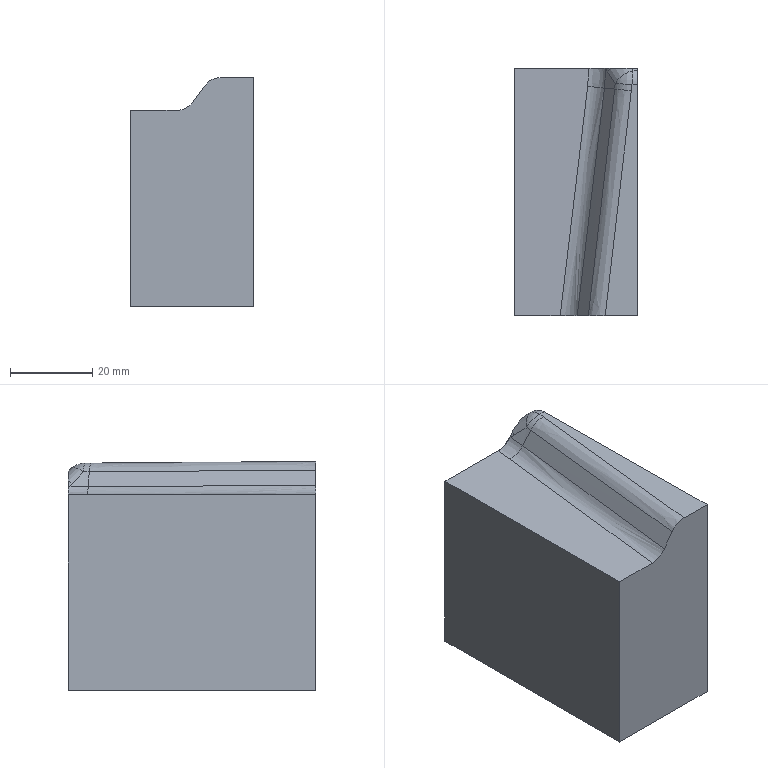Part | NX | features solid 2 | 1 solid | 19 faces | box 30 x 60 x 55.625 mm | volume 90245 mm3 | spline 14 | plane 5
STEP:
#1=CARTESIAN_POINT('',(-115.283,294.27,47.484));
#2=VERTEX_POINT('',#1);
#3=CARTESIAN_POINT('',(-133.378,294.27,47.551));
#4=VERTEX_POINT('',#3);
#5=CARTESIAN_POINT('',(-103.184,294.27,47.439));
#6=DIRECTION('',(-1.,0.,0.003698));
#7=VECTOR('',#6,1000.);
#8=LINE('',#5,#7);
#9=EDGE_CURVE('',#2,#4,#8,.T.);
#10=ORIENTED_EDGE('',*,*,#9,.F.);
#11=CARTESIAN_POINT('',(-111.203,294.27,49.568));
#12=VERTEX_POINT('',#11);
#13=CARTESIAN_POINT('',(-115.284,294.27,47.484));
#14=CARTESIAN_POINT('',(-113.684,294.27,47.478));
#15=CARTESIAN_POINT('',(-112.137,294.27,48.268));
#16=CARTESIAN_POINT('',(-111.203,294.27,49.568));
#17=B_SPLINE_CURVE_WITH_KNOTS('',3,(#13,#14,#15,#16),.UNSPECIFIED.,.F.,.F.,(4,4),(0.,0.004736),.UNSPECIFIED.);
#18=EDGE_CURVE('',#2,#12,#17,.T.);
#19=ORIENTED_EDGE('',*,*,#18,.T.);
#20=CARTESIAN_POINT('',(-110.093,294.27,50.867));
#21=VERTEX_POINT('',#20);
#22=CARTESIAN_POINT('',(-110.093,294.27,50.867));
#23=CARTESIAN_POINT('',(-110.496,294.27,50.461));
#24=CARTESIAN_POINT('',(-110.87,294.27,50.032));
#25=CARTESIAN_POINT('',(-111.203,294.27,49.568));
#26=B_SPLINE_CURVE_WITH_KNOTS('',3,(#22,#23,#24,#25),.UNSPECIFIED.,.F.,.F.,(4,4),(0.,0.001709),.UNSPECIFIED.);
#27=EDGE_CURVE('',#21,#12,#26,.T.);
#28=ORIENTED_EDGE('',*,*,#27,.F.);
#29=CARTESIAN_POINT('',(-104.912,294.27,53.297));
#30=VERTEX_POINT('',#29);
#31=CARTESIAN_POINT('',(-110.093,294.27,50.867));
#32=CARTESIAN_POINT('',(-109.399,294.27,51.567));
#33=CARTESIAN_POINT('',(-107.835,294.27,52.779));
#34=CARTESIAN_POINT('',(-105.906,294.27,53.356));
#35=CARTESIAN_POINT('',(-104.912,294.27,53.297));
#36=B_SPLINE_CURVE_WITH_KNOTS('',3,(#31,#32,#33,#34,#35),.UNSPECIFIED.,.F.,.F.,(4,1,4),(0.,0.00295,0.0059),.UNSPECIFIED.);
#37=EDGE_CURVE('',#21,#30,#36,.T.);
#38=ORIENTED_EDGE('',*,*,#37,.T.);
#39=CARTESIAN_POINT('',(-103.378,294.27,53.207));
#40=VERTEX_POINT('',#39);
#41=CARTESIAN_POINT('',(-99.969,294.27,53.007));
#42=DIRECTION('',(0.9983,0.,-0.05867));
#43=VECTOR('',#42,1000.);
#44=LINE('',#41,#43);
#45=EDGE_CURVE('',#30,#40,#44,.T.);
#46=ORIENTED_EDGE('',*,*,#45,.T.);
#47=CARTESIAN_POINT('',(-103.378,294.27,0.));
#48=VERTEX_POINT('',#47);
#49=CARTESIAN_POINT('',(-103.378,294.27,-5.));
#50=DIRECTION('',(0.,0.,-1.));
#51=VECTOR('',#50,1000.);
#52=LINE('',#49,#51);
#53=EDGE_CURVE('',#48,#40,#52,.F.);
#54=ORIENTED_EDGE('',*,*,#53,.F.);
#55=CARTESIAN_POINT('',(-133.378,294.27,0.));
#56=VERTEX_POINT('',#55);
#57=CARTESIAN_POINT('',(-103.378,294.27,0.));
#58=DIRECTION('',(1.,0.,0.));
#59=VECTOR('',#58,1000.);
#60=LINE('',#57,#59);
#61=EDGE_CURVE('',#48,#56,#60,.F.);
#62=ORIENTED_EDGE('',*,*,#61,.T.);
#63=CARTESIAN_POINT('',(-133.378,294.27,-5.));
#64=DIRECTION('',(0.,0.,-1.));
#65=VECTOR('',#64,1000.);
#66=LINE('',#63,#65);
#67=EDGE_CURVE('',#56,#4,#66,.F.);
#68=ORIENTED_EDGE('',*,*,#67,.T.);
#69=EDGE_LOOP('',(#10,#19,#28,#38,#46,#54,#62,#68));
#70=FACE_BOUND('',#69,.T.);
#71=CARTESIAN_POINT('',(-103.378,294.27,-5.));
#72=DIRECTION('',(0.,1.,0.));
#73=DIRECTION('',(-1.,0.,0.));
#74=AXIS2_PLACEMENT_3D('',#71,#72,#73);
#75=PLANE('',#74);
#76=ADVANCED_FACE('',(#70),#75,.T.);
#77=CARTESIAN_POINT('',(-133.378,234.27,47.656));
#78=VERTEX_POINT('',#77);
#79=CARTESIAN_POINT('',(-122.215,234.27,47.614));
#80=VERTEX_POINT('',#79);
#81=CARTESIAN_POINT('',(-103.184,234.27,47.544));
#82=DIRECTION('',(-1.,0.,0.003698));
#83=VECTOR('',#82,1000.);
#84=LINE('',#81,#83);
#85=EDGE_CURVE('',#78,#80,#84,.F.);
#86=ORIENTED_EDGE('',*,*,#85,.F.);
#87=CARTESIAN_POINT('',(-133.378,234.27,0.));
#88=VERTEX_POINT('',#87);
#89=CARTESIAN_POINT('',(-133.378,234.27,-5.));
#90=DIRECTION('',(0.,0.,-1.));
#91=VECTOR('',#90,1000.);
#92=LINE('',#89,#91);
#93=EDGE_CURVE('',#88,#78,#92,.F.);
#94=ORIENTED_EDGE('',*,*,#93,.F.);
#95=CARTESIAN_POINT('',(-103.378,234.27,0.));
#96=VERTEX_POINT('',#95);
#97=CARTESIAN_POINT('',(-103.378,234.27,0.));
#98=DIRECTION('',(-1.,0.,0.));
#99=VECTOR('',#98,1000.);
#100=LINE('',#97,#99);
#101=EDGE_CURVE('',#96,#88,#100,.T.);
#102=ORIENTED_EDGE('',*,*,#101,.F.);
#103=CARTESIAN_POINT('',(-103.378,234.27,55.625));
#104=VERTEX_POINT('',#103);
#105=CARTESIAN_POINT('',(-103.378,234.27,-5.));
#106=DIRECTION('',(0.,0.,-1.));
#107=VECTOR('',#106,1000.);
#108=LINE('',#105,#107);
#109=EDGE_CURVE('',#96,#104,#108,.F.);
#110=ORIENTED_EDGE('',*,*,#109,.T.);
#111=CARTESIAN_POINT('',(-111.283,234.27,55.625));
#112=VERTEX_POINT('',#111);
#113=CARTESIAN_POINT('',(-103.378,234.27,55.625));
#114=DIRECTION('',(1.,0.,0.));
#115=VECTOR('',#114,1000.);
#116=LINE('',#113,#115);
#117=EDGE_CURVE('',#104,#112,#116,.F.);
#118=ORIENTED_EDGE('',*,*,#117,.T.);
#119=CARTESIAN_POINT('',(-115.39,234.27,53.514));
#120=VERTEX_POINT('',#119);
#121=CARTESIAN_POINT('',(-111.283,234.27,55.625));
#122=CARTESIAN_POINT('',(-112.896,234.27,55.625));
#123=CARTESIAN_POINT('',(-114.454,234.27,54.829));
#124=CARTESIAN_POINT('',(-115.39,234.27,53.514));
#125=B_SPLINE_CURVE_WITH_KNOTS('',3,(#121,#122,#123,#124),.UNSPECIFIED.,.F.,.F.,(4,4),(0.,0.004803),.UNSPECIFIED.);
#126=EDGE_CURVE('',#112,#120,#125,.T.);
#127=ORIENTED_EDGE('',*,*,#126,.T.);
#128=CARTESIAN_POINT('',(-118.085,234.27,49.728));
#129=VERTEX_POINT('',#128);
#130=CARTESIAN_POINT('',(-138.995,234.27,20.355));
#131=DIRECTION('',(-0.5799,0.,-0.8147));
#132=VECTOR('',#131,1000.);
#133=LINE('',#130,#132);
#134=EDGE_CURVE('',#129,#120,#133,.F.);
#135=ORIENTED_EDGE('',*,*,#134,.F.);
#136=CARTESIAN_POINT('',(-122.215,234.27,47.614));
#137=CARTESIAN_POINT('',(-120.594,234.27,47.608));
#138=CARTESIAN_POINT('',(-119.026,234.27,48.407));
#139=CARTESIAN_POINT('',(-118.085,234.27,49.728));
#140=B_SPLINE_CURVE_WITH_KNOTS('',3,(#136,#137,#138,#139),.UNSPECIFIED.,.F.,.F.,(4,4),(0.,0.004827),.UNSPECIFIED.);
#141=EDGE_CURVE('',#80,#129,#140,.T.);
#142=ORIENTED_EDGE('',*,*,#141,.F.);
#143=EDGE_LOOP('',(#86,#94,#102,#110,#118,#127,#135,#142));
#144=FACE_BOUND('',#143,.T.);
#145=CARTESIAN_POINT('',(-103.378,234.27,-5.));
#146=DIRECTION('',(0.,1.,0.));
#147=DIRECTION('',(-1.,0.,0.));
#148=AXIS2_PLACEMENT_3D('',#145,#146,#147);
#149=PLANE('',#148);
#150=ADVANCED_FACE('',(#144),#149,.F.);
#151=CARTESIAN_POINT('',(-133.378,294.362,47.551));
#152=DIRECTION('',(0.,-1.,0.00175));
#153=VECTOR('',#152,1000.);
#154=LINE('',#151,#153);
#155=EDGE_CURVE('',#4,#78,#154,.T.);
#156=ORIENTED_EDGE('',*,*,#155,.F.);
#157=ORIENTED_EDGE('',*,*,#67,.F.);
#158=CARTESIAN_POINT('',(-133.378,294.27,0.));
#159=DIRECTION('',(0.,1.,0.));
#160=VECTOR('',#159,1000.);
#161=LINE('',#158,#160);
#162=EDGE_CURVE('',#56,#88,#161,.F.);
#163=ORIENTED_EDGE('',*,*,#162,.T.);
#164=ORIENTED_EDGE('',*,*,#93,.T.);
#165=EDGE_LOOP('',(#156,#157,#163,#164));
#166=FACE_BOUND('',#165,.T.);
#167=CARTESIAN_POINT('',(-133.378,294.27,-5.));
#168=DIRECTION('',(-1.,0.,0.));
#169=DIRECTION('',(0.,-1.,0.));
#170=AXIS2_PLACEMENT_3D('',#167,#168,#169);
#171=PLANE('',#170);
#172=ADVANCED_FACE('',(#166),#171,.T.);
#173=CARTESIAN_POINT('',(-103.378,293.627,53.826));
#174=VERTEX_POINT('',#173);
#175=CARTESIAN_POINT('',(-103.378,290.188,55.224));
#176=VERTEX_POINT('',#175);
#177=CARTESIAN_POINT('',(-103.378,293.627,53.826));
#178=CARTESIAN_POINT('',(-103.378,292.707,54.71));
#179=CARTESIAN_POINT('',(-103.378,291.464,55.215));
#180=CARTESIAN_POINT('',(-103.378,290.188,55.224));
#181=B_SPLINE_CURVE_WITH_KNOTS('',3,(#177,#178,#179,#180),.UNSPECIFIED.,.F.,.F.,(4,4),(0.,0.003809),.UNSPECIFIED.);
#182=EDGE_CURVE('',#174,#176,#181,.T.);
#183=ORIENTED_EDGE('',*,*,#182,.T.);
#184=CARTESIAN_POINT('',(-103.378,294.703,55.192));
#185=DIRECTION('',(0.,1.,-0.007178));
#186=VECTOR('',#185,1000.);
#187=LINE('',#184,#186);
#188=EDGE_CURVE('',#176,#104,#187,.F.);
#189=ORIENTED_EDGE('',*,*,#188,.T.);
#190=ORIENTED_EDGE('',*,*,#109,.F.);
#191=CARTESIAN_POINT('',(-103.378,294.27,0.));
#192=DIRECTION('',(0.,-1.,0.));
#193=VECTOR('',#192,1000.);
#194=LINE('',#191,#193);
#195=EDGE_CURVE('',#48,#96,#194,.T.);
#196=ORIENTED_EDGE('',*,*,#195,.F.);
#197=ORIENTED_EDGE('',*,*,#53,.T.);
#198=CARTESIAN_POINT('',(-103.378,323.351,25.253));
#199=DIRECTION('',(0.,0.7209,-0.693));
#200=VECTOR('',#199,1000.);
#201=LINE('',#198,#200);
#202=EDGE_CURVE('',#40,#174,#201,.F.);
#203=ORIENTED_EDGE('',*,*,#202,.T.);
#204=EDGE_LOOP('',(#183,#189,#190,#196,#197,#203));
#205=FACE_BOUND('',#204,.T.);
#206=CARTESIAN_POINT('',(-103.378,294.27,-5.));
#207=DIRECTION('',(-1.,0.,0.));
#208=DIRECTION('',(0.,-1.,0.));
#209=AXIS2_PLACEMENT_3D('',#206,#207,#208);
#210=PLANE('',#209);
#211=ADVANCED_FACE('',(#205),#210,.F.);
#212=ORIENTED_EDGE('',*,*,#101,.T.);
#213=ORIENTED_EDGE('',*,*,#162,.F.);
#214=ORIENTED_EDGE('',*,*,#61,.F.);
#215=ORIENTED_EDGE('',*,*,#195,.T.);
#216=EDGE_LOOP('',(#212,#213,#214,#215));
#217=FACE_BOUND('',#216,.T.);
#218=CARTESIAN_POINT('',(-103.378,294.27,0.));
#219=DIRECTION('',(0.,0.,1.));
#220=DIRECTION('',(1.,0.,0.));
#221=AXIS2_PLACEMENT_3D('',#218,#219,#220);
#222=PLANE('',#221);
#223=ADVANCED_FACE('',(#217),#222,.F.);
#224=CARTESIAN_POINT('',(-115.285,294.158,47.484));
#225=VERTEX_POINT('',#224);
#226=CARTESIAN_POINT('',(-115.284,294.27,47.484));
#227=CARTESIAN_POINT('',(-115.284,294.233,47.484));
#228=CARTESIAN_POINT('',(-115.285,294.195,47.484));
#229=CARTESIAN_POINT('',(-115.285,294.158,47.484));
#230=B_SPLINE_CURVE_WITH_KNOTS('',3,(#226,#227,#228,#229),.UNSPECIFIED.,.F.,.F.,(4,4),(0.965,1.),.UNSPECIFIED.);
#231=EDGE_CURVE('',#2,#225,#230,.T.);
#232=ORIENTED_EDGE('',*,*,#231,.T.);
#233=CARTESIAN_POINT('',(-111.18,294.144,49.603));
#234=VERTEX_POINT('',#233);
#235=CARTESIAN_POINT('',(-115.285,294.158,47.484));
#236=CARTESIAN_POINT('',(-113.684,294.151,47.478));
#237=CARTESIAN_POINT('',(-112.102,294.146,48.295));
#238=CARTESIAN_POINT('',(-111.18,294.144,49.603));
#239=B_SPLINE_CURVE_WITH_KNOTS('',3,(#235,#236,#237,#238),.UNSPECIFIED.,.F.,.F.,(4,4),(0.,1.),.UNSPECIFIED.);
#240=EDGE_CURVE('',#234,#225,#239,.F.);
#241=ORIENTED_EDGE('',*,*,#240,.F.);
#242=CARTESIAN_POINT('',(-111.18,294.144,49.603));
#243=CARTESIAN_POINT('',(-111.188,294.186,49.591));
#244=CARTESIAN_POINT('',(-111.196,294.228,49.58));
#245=CARTESIAN_POINT('',(-111.203,294.27,49.568));
#246=B_SPLINE_CURVE_WITH_KNOTS('',3,(#242,#243,#244,#245),.UNSPECIFIED.,.F.,.F.,(4,4),(0.,0.04789),.UNSPECIFIED.);
#247=EDGE_CURVE('',#234,#12,#246,.T.);
#248=ORIENTED_EDGE('',*,*,#247,.T.);
#249=ORIENTED_EDGE('',*,*,#18,.F.);
#250=EDGE_LOOP('',(#232,#241,#248,#249));
#251=FACE_BOUND('',#250,.T.);
#252=CARTESIAN_POINT('',(-115.283,294.313,47.484));
#253=CARTESIAN_POINT('',(-114.332,294.302,47.48));
#254=CARTESIAN_POINT('',(-113.379,294.292,47.703));
#255=CARTESIAN_POINT('',(-112.498,294.283,48.154));
#256=CARTESIAN_POINT('',(-111.759,294.276,48.795));
#257=CARTESIAN_POINT('',(-111.204,294.271,49.568));
#258=CARTESIAN_POINT('',(-115.284,294.282,47.484));
#259=CARTESIAN_POINT('',(-114.33,294.273,47.48));
#260=CARTESIAN_POINT('',(-113.376,294.264,47.704));
#261=CARTESIAN_POINT('',(-112.493,294.256,48.156));
#262=CARTESIAN_POINT('',(-111.754,294.25,48.799));
#263=CARTESIAN_POINT('',(-111.199,294.246,49.575));
#264=CARTESIAN_POINT('',(-115.284,294.251,47.484));
#265=CARTESIAN_POINT('',(-114.329,294.243,47.48));
#266=CARTESIAN_POINT('',(-113.373,294.235,47.705));
#267=CARTESIAN_POINT('',(-112.489,294.229,48.158));
#268=CARTESIAN_POINT('',(-111.749,294.224,48.804));
#269=CARTESIAN_POINT('',(-111.194,294.22,49.582));
#270=CARTESIAN_POINT('',(-115.284,294.22,47.484));
#271=CARTESIAN_POINT('',(-114.327,294.213,47.48));
#272=CARTESIAN_POINT('',(-113.37,294.207,47.706));
#273=CARTESIAN_POINT('',(-112.484,294.202,48.161));
#274=CARTESIAN_POINT('',(-111.743,294.198,48.809));
#275=CARTESIAN_POINT('',(-111.189,294.195,49.589));
#276=CARTESIAN_POINT('',(-115.285,294.189,47.484));
#277=CARTESIAN_POINT('',(-114.326,294.183,47.48));
#278=CARTESIAN_POINT('',(-113.366,294.179,47.707));
#279=CARTESIAN_POINT('',(-112.48,294.174,48.163));
#280=CARTESIAN_POINT('',(-111.738,294.171,48.813));
#281=CARTESIAN_POINT('',(-111.185,294.17,49.596));
#282=CARTESIAN_POINT('',(-115.285,294.158,47.484));
#283=CARTESIAN_POINT('',(-114.324,294.154,47.481));
#284=CARTESIAN_POINT('',(-113.363,294.15,47.708));
#285=CARTESIAN_POINT('',(-112.475,294.147,48.166));
#286=CARTESIAN_POINT('',(-111.733,294.145,48.818));
#287=CARTESIAN_POINT('',(-111.18,294.144,49.603));
#288=B_SPLINE_SURFACE_WITH_KNOTS('',5,5,((#252,#253,#254,#255,#256,#257),(#258,#259,#260,#261,#262,#263),(#264,#265,#266,#267,#268,#269),(#270,#271,#272,#273,#274,#275),(#276,#277,#278,#279,#280,#281),(#282,#283,#284,#285,#286,#287)),.UNSPECIFIED.,.F.,.F.,.F.,(6,6),(6,6),(0.9518,1.),(0.,1.),.PIECEWISE_BEZIER_KNOTS.);
#289=ADVANCED_FACE('',(#251),#288,.T.);
#290=ORIENTED_EDGE('',*,*,#27,.T.);
#291=ORIENTED_EDGE('',*,*,#247,.F.);
#292=CARTESIAN_POINT('',(-110.699,293.366,50.301));
#293=VERTEX_POINT('',#292);
#294=CARTESIAN_POINT('',(-110.699,293.366,50.301));
#295=CARTESIAN_POINT('',(-110.866,293.608,50.056));
#296=CARTESIAN_POINT('',(-111.027,293.867,49.822));
#297=CARTESIAN_POINT('',(-111.18,294.144,49.603));
#298=B_SPLINE_CURVE_WITH_KNOTS('',3,(#294,#295,#296,#297),.UNSPECIFIED.,.F.,.F.,(4,4),(0.,1.),.UNSPECIFIED.);
#299=EDGE_CURVE('',#293,#234,#298,.T.);
#300=ORIENTED_EDGE('',*,*,#299,.F.);
#301=CARTESIAN_POINT('',(-110.093,294.27,50.867));
#302=CARTESIAN_POINT('',(-110.332,293.976,50.711));
#303=CARTESIAN_POINT('',(-110.536,293.671,50.52));
#304=CARTESIAN_POINT('',(-110.699,293.366,50.301));
#305=B_SPLINE_CURVE_WITH_KNOTS('',3,(#301,#302,#303,#304),.UNSPECIFIED.,.F.,.F.,(4,4),(0.7889,1.),.UNSPECIFIED.);
#306=EDGE_CURVE('',#21,#293,#305,.T.);
#307=ORIENTED_EDGE('',*,*,#306,.F.);
#308=EDGE_LOOP('',(#290,#291,#300,#307));
#309=FACE_BOUND('',#308,.T.);
#310=CARTESIAN_POINT('',(-110.593,295.007,50.184));
#311=CARTESIAN_POINT('',(-110.742,294.857,50.072));
#312=CARTESIAN_POINT('',(-110.881,294.704,49.95));
#313=CARTESIAN_POINT('',(-111.009,294.55,49.818));
#314=CARTESIAN_POINT('',(-111.126,294.395,49.678));
#315=CARTESIAN_POINT('',(-111.232,294.239,49.529));
#316=CARTESIAN_POINT('',(-110.498,294.849,50.312));
#317=CARTESIAN_POINT('',(-110.646,294.693,50.203));
#318=CARTESIAN_POINT('',(-110.783,294.534,50.085));
#319=CARTESIAN_POINT('',(-110.911,294.374,49.956));
#320=CARTESIAN_POINT('',(-111.027,294.213,49.819));
#321=CARTESIAN_POINT('',(-111.131,294.052,49.673));
#322=CARTESIAN_POINT('',(-110.399,294.697,50.445));
#323=CARTESIAN_POINT('',(-110.546,294.535,50.34));
#324=CARTESIAN_POINT('',(-110.683,294.371,50.225));
#325=CARTESIAN_POINT('',(-110.809,294.204,50.1));
#326=CARTESIAN_POINT('',(-110.924,294.037,49.965));
#327=CARTESIAN_POINT('',(-111.027,293.87,49.823));
#328=CARTESIAN_POINT('',(-110.298,294.55,50.583));
#329=CARTESIAN_POINT('',(-110.444,294.383,50.481));
#330=CARTESIAN_POINT('',(-110.58,294.213,50.37));
#331=CARTESIAN_POINT('',(-110.705,294.041,50.248));
#332=CARTESIAN_POINT('',(-110.819,293.869,50.117));
#333=CARTESIAN_POINT('',(-110.92,293.695,49.977));
#334=CARTESIAN_POINT('',(-110.195,294.41,50.724));
#335=CARTESIAN_POINT('',(-110.34,294.237,50.627));
#336=CARTESIAN_POINT('',(-110.475,294.062,50.519));
#337=CARTESIAN_POINT('',(-110.599,293.885,50.401));
#338=CARTESIAN_POINT('',(-110.711,293.706,50.273));
#339=CARTESIAN_POINT('',(-110.811,293.527,50.137));
#340=CARTESIAN_POINT('',(-110.089,294.276,50.87));
#341=CARTESIAN_POINT('',(-110.234,294.098,50.776));
#342=CARTESIAN_POINT('',(-110.368,293.917,50.672));
#343=CARTESIAN_POINT('',(-110.49,293.734,50.557));
#344=CARTESIAN_POINT('',(-110.601,293.55,50.433));
#345=CARTESIAN_POINT('',(-110.699,293.366,50.301));
#346=B_SPLINE_SURFACE_WITH_KNOTS('',5,5,((#310,#311,#312,#313,#314,#315),(#316,#317,#318,#319,#320,#321),(#322,#323,#324,#325,#326,#327),(#328,#329,#330,#331,#332,#333),(#334,#335,#336,#337,#338,#339),(#340,#341,#342,#343,#344,#345)),.UNSPECIFIED.,.F.,.F.,.F.,(6,6),(6,6),(0.6827,1.),(0.7877,1.),.PIECEWISE_BEZIER_KNOTS.);
#347=ADVANCED_FACE('',(#309),#346,.F.);
#348=ORIENTED_EDGE('',*,*,#306,.T.);
#349=CARTESIAN_POINT('',(-108.861,290.595,53.109));
#350=VERTEX_POINT('',#349);
#351=CARTESIAN_POINT('',(-110.699,293.366,50.301));
#352=CARTESIAN_POINT('',(-110.064,292.449,51.23));
#353=CARTESIAN_POINT('',(-109.452,291.526,52.166));
#354=CARTESIAN_POINT('',(-108.863,290.595,53.111));
#355=B_SPLINE_CURVE_WITH_KNOTS('',3,(#351,#352,#353,#354),.UNSPECIFIED.,.F.,.F.,(4,4),(0.,1.),.UNSPECIFIED.);
#356=EDGE_CURVE('',#350,#293,#355,.F.);
#357=ORIENTED_EDGE('',*,*,#356,.F.);
#358=CARTESIAN_POINT('',(-104.584,293.701,53.825));
#359=VERTEX_POINT('',#358);
#360=CARTESIAN_POINT('',(-108.863,290.595,53.111));
#361=CARTESIAN_POINT('',(-108.047,291.971,54.091));
#362=CARTESIAN_POINT('',(-106.313,293.229,54.38));
#363=CARTESIAN_POINT('',(-104.584,293.701,53.825));
#364=B_SPLINE_CURVE_WITH_KNOTS('',3,(#360,#361,#362,#363),.UNSPECIFIED.,.F.,.F.,(4,4),(0.,1.),.UNSPECIFIED.);
#365=EDGE_CURVE('',#350,#359,#364,.T.);
#366=ORIENTED_EDGE('',*,*,#365,.T.);
#367=CARTESIAN_POINT('',(-104.584,293.701,53.825));
#368=CARTESIAN_POINT('',(-104.693,293.891,53.649));
#369=CARTESIAN_POINT('',(-104.802,294.081,53.473));
#370=CARTESIAN_POINT('',(-104.912,294.27,53.297));
#371=B_SPLINE_CURVE_WITH_KNOTS('',3,(#367,#368,#369,#370),.UNSPECIFIED.,.F.,.F.,(4,4),(0.,0.1866),.UNSPECIFIED.);
#372=EDGE_CURVE('',#30,#359,#371,.F.);
#373=ORIENTED_EDGE('',*,*,#372,.F.);
#374=ORIENTED_EDGE('',*,*,#37,.F.);
#375=EDGE_LOOP('',(#348,#357,#366,#373,#374));
#376=FACE_BOUND('',#375,.T.);
#377=CARTESIAN_POINT('',(-104.584,293.701,53.825));
#378=CARTESIAN_POINT('',(-105.621,293.418,54.158));
#379=CARTESIAN_POINT('',(-106.672,292.916,54.263));
#380=CARTESIAN_POINT('',(-107.626,292.223,54.104));
#381=CARTESIAN_POINT('',(-108.373,291.421,53.699));
#382=CARTESIAN_POINT('',(-108.863,290.595,53.111));
#383=CARTESIAN_POINT('',(-104.933,294.312,53.258));
#384=CARTESIAN_POINT('',(-105.974,294.021,53.599));
#385=CARTESIAN_POINT('',(-107.029,293.508,53.709));
#386=CARTESIAN_POINT('',(-107.986,292.803,53.549));
#387=CARTESIAN_POINT('',(-108.732,291.988,53.139));
#388=CARTESIAN_POINT('',(-109.216,291.154,52.544));
#389=CARTESIAN_POINT('',(-105.29,294.921,52.695));
#390=CARTESIAN_POINT('',(-106.335,294.622,53.043));
#391=CARTESIAN_POINT('',(-107.394,294.098,53.157));
#392=CARTESIAN_POINT('',(-108.353,293.38,52.997));
#393=CARTESIAN_POINT('',(-109.097,292.553,52.582));
#394=CARTESIAN_POINT('',(-109.576,291.71,51.98));
#395=CARTESIAN_POINT('',(-105.654,295.527,52.133));
#396=CARTESIAN_POINT('',(-106.703,295.22,52.489));
#397=CARTESIAN_POINT('',(-107.766,294.685,52.608));
#398=CARTESIAN_POINT('',(-108.727,293.954,52.447));
#399=CARTESIAN_POINT('',(-109.47,293.116,52.028));
#400=CARTESIAN_POINT('',(-109.944,292.264,51.418));
#401=CARTESIAN_POINT('',(-106.025,296.131,51.574));
#402=CARTESIAN_POINT('',(-107.078,295.817,51.938));
#403=CARTESIAN_POINT('',(-108.146,295.27,52.061));
#404=CARTESIAN_POINT('',(-109.109,294.527,51.9));
#405=CARTESIAN_POINT('',(-109.85,293.676,51.476));
#406=CARTESIAN_POINT('',(-110.318,292.816,50.858));
#407=CARTESIAN_POINT('',(-106.404,296.732,51.018));
#408=CARTESIAN_POINT('',(-107.461,296.41,51.39));
#409=CARTESIAN_POINT('',(-108.532,295.853,51.517));
#410=CARTESIAN_POINT('',(-109.498,295.097,51.355));
#411=CARTESIAN_POINT('',(-110.237,294.235,50.926));
#412=CARTESIAN_POINT('',(-110.699,293.366,50.301));
#413=B_SPLINE_SURFACE_WITH_KNOTS('',5,5,((#377,#378,#379,#380,#381,#382),(#383,#384,#385,#386,#387,#388),(#389,#390,#391,#392,#393,#394),(#395,#396,#397,#398,#399,#400),(#401,#402,#403,#404,#405,#406),(#407,#408,#409,#410,#411,#412)),.UNSPECIFIED.,.F.,.F.,.F.,(6,6),(6,6),(0.,1.),(0.,1.),.PIECEWISE_BEZIER_KNOTS.);
#414=ADVANCED_FACE('',(#376),#413,.T.);
#415=ORIENTED_EDGE('',*,*,#372,.T.);
#416=CARTESIAN_POINT('',(-104.584,293.701,53.825));
#417=CARTESIAN_POINT('',(-104.182,293.677,53.825));
#418=CARTESIAN_POINT('',(-103.78,293.652,53.825));
#419=CARTESIAN_POINT('',(-103.378,293.627,53.826));
#420=B_SPLINE_CURVE_WITH_KNOTS('',3,(#416,#417,#418,#419),.UNSPECIFIED.,.F.,.F.,(4,4),(0.,0.02048),.UNSPECIFIED.);
#421=EDGE_CURVE('',#359,#174,#420,.T.);
#422=ORIENTED_EDGE('',*,*,#421,.T.);
#423=ORIENTED_EDGE('',*,*,#202,.F.);
#424=ORIENTED_EDGE('',*,*,#45,.F.);
#425=EDGE_LOOP('',(#415,#422,#423,#424));
#426=FACE_BOUND('',#425,.T.);
#427=CARTESIAN_POINT('',(-104.922,294.32,53.251));
#428=CARTESIAN_POINT('',(-103.378,294.274,53.203));
#429=CARTESIAN_POINT('',(-104.922,293.669,53.876));
#430=CARTESIAN_POINT('',(-103.378,293.623,53.829));
#431=B_SPLINE_SURFACE_WITH_KNOTS('',1,1,((#427,#428),(#429,#430)),.PLANE_SURF.,.F.,.F.,.F.,(2,2),(2,2),(0.551,0.6661),(0.03004,0.05514),.PIECEWISE_BEZIER_KNOTS.);
#432=ADVANCED_FACE('',(#426),#431,.T.);
#433=ORIENTED_EDGE('',*,*,#421,.F.);
#434=CARTESIAN_POINT('',(-104.796,290.275,55.222));
#435=VERTEX_POINT('',#434);
#436=CARTESIAN_POINT('',(-104.796,290.275,55.223));
#437=CARTESIAN_POINT('',(-104.72,291.509,55.215));
#438=CARTESIAN_POINT('',(-104.639,292.813,54.682));
#439=CARTESIAN_POINT('',(-104.584,293.701,53.825));
#440=B_SPLINE_CURVE_WITH_KNOTS('',3,(#436,#437,#438,#439),.UNSPECIFIED.,.F.,.F.,(4,4),(0.,1.),.UNSPECIFIED.);
#441=EDGE_CURVE('',#435,#359,#440,.T.);
#442=ORIENTED_EDGE('',*,*,#441,.F.);
#443=CARTESIAN_POINT('',(-103.378,290.188,55.224));
#444=CARTESIAN_POINT('',(-103.851,290.217,55.224));
#445=CARTESIAN_POINT('',(-104.323,290.246,55.224));
#446=CARTESIAN_POINT('',(-104.796,290.275,55.223));
#447=B_SPLINE_CURVE_WITH_KNOTS('',3,(#443,#444,#445,#446),.UNSPECIFIED.,.F.,.F.,(4,4),(0.7806,1.),.UNSPECIFIED.);
#448=EDGE_CURVE('',#176,#435,#447,.T.);
#449=ORIENTED_EDGE('',*,*,#448,.F.);
#450=ORIENTED_EDGE('',*,*,#182,.F.);
#451=EDGE_LOOP('',(#433,#442,#449,#450));
#452=FACE_BOUND('',#451,.T.);
#453=CARTESIAN_POINT('',(-104.796,290.275,55.223));
#454=CARTESIAN_POINT('',(-103.37,290.188,55.224));
#455=CARTESIAN_POINT('',(-104.716,291.57,55.214));
#456=CARTESIAN_POINT('',(-103.29,291.482,55.215));
#457=CARTESIAN_POINT('',(-104.642,292.769,54.725));
#458=CARTESIAN_POINT('',(-103.216,292.681,54.725));
#459=CARTESIAN_POINT('',(-104.584,293.701,53.825));
#460=CARTESIAN_POINT('',(-103.158,293.614,53.826));
#461=(BOUNDED_SURFACE()B_SPLINE_SURFACE(3,1,((#453,#454),(#455,#456),(#457,#458),(#459,#460)),.CYLINDRICAL_SURF.,.F.,.F.,.F.)B_SPLINE_SURFACE_WITH_KNOTS((4,4),(2,2),(0.,1.),(0.,0.02422),.PIECEWISE_BEZIER_KNOTS.)GEOMETRIC_REPRESENTATION_ITEM()RATIONAL_B_SPLINE_SURFACE(((1.,1.),(0.9525,0.9525),(0.9525,0.9525),(1.,1.)))REPRESENTATION_ITEM('')SURFACE());
#462=ADVANCED_FACE('',(#452),#461,.F.);
#463=ORIENTED_EDGE('',*,*,#141,.T.);
#464=CARTESIAN_POINT('',(-111.474,289.44,49.607));
#465=VERTEX_POINT('',#464);
#466=CARTESIAN_POINT('',(-118.085,234.27,49.728));
#467=CARTESIAN_POINT('',(-115.882,252.66,49.687));
#468=CARTESIAN_POINT('',(-113.678,271.05,49.647));
#469=CARTESIAN_POINT('',(-111.474,289.44,49.607));
#470=B_SPLINE_CURVE_WITH_KNOTS('',3,(#466,#467,#468,#469),.UNSPECIFIED.,.F.,.F.,(4,4),(0.4119,1.),.UNSPECIFIED.);
#471=EDGE_CURVE('',#465,#129,#470,.F.);
#472=ORIENTED_EDGE('',*,*,#471,.F.);
#473=CARTESIAN_POINT('',(-115.546,289.923,47.492));
#474=VERTEX_POINT('',#473);
#475=CARTESIAN_POINT('',(-111.474,289.44,49.607));
#476=CARTESIAN_POINT('',(-111.915,289.491,48.979));
#477=CARTESIAN_POINT('',(-113.159,289.638,47.862));
#478=CARTESIAN_POINT('',(-114.783,289.832,47.49));
#479=CARTESIAN_POINT('',(-115.546,289.923,47.492));
#480=B_SPLINE_CURVE_WITH_KNOTS('',3,(#475,#476,#477,#478,#479),.UNSPECIFIED.,.F.,.F.,(4,1,4),(0.,0.5,1.),.UNSPECIFIED.);
#481=EDGE_CURVE('',#474,#465,#480,.F.);
#482=ORIENTED_EDGE('',*,*,#481,.F.);
#483=CARTESIAN_POINT('',(-115.546,289.923,47.492));
#484=CARTESIAN_POINT('',(-117.769,271.372,47.533));
#485=CARTESIAN_POINT('',(-119.992,252.821,47.574));
#486=CARTESIAN_POINT('',(-122.215,234.27,47.614));
#487=B_SPLINE_CURVE_WITH_KNOTS('',3,(#483,#484,#485,#486),.UNSPECIFIED.,.F.,.F.,(4,4),(0.,0.5932),.UNSPECIFIED.);
#488=EDGE_CURVE('',#474,#80,#487,.T.);
#489=ORIENTED_EDGE('',*,*,#488,.T.);
#490=EDGE_LOOP('',(#463,#472,#482,#489));
#491=FACE_BOUND('',#490,.T.);
#492=CARTESIAN_POINT('',(-118.183,233.453,49.73));
#493=CARTESIAN_POINT('',(-111.474,289.44,49.607));
#494=CARTESIAN_POINT('',(-119.137,233.564,48.372));
#495=CARTESIAN_POINT('',(-112.427,289.551,48.249));
#496=CARTESIAN_POINT('',(-120.604,233.739,47.609));
#497=CARTESIAN_POINT('',(-113.895,289.725,47.487));
#498=CARTESIAN_POINT('',(-122.255,233.937,47.615));
#499=CARTESIAN_POINT('',(-115.546,289.923,47.492));
#500=(BOUNDED_SURFACE()B_SPLINE_SURFACE(3,1,((#492,#493),(#494,#495),(#496,#497),(#498,#499)),.CYLINDRICAL_SURF.,.F.,.F.,.F.)B_SPLINE_SURFACE_WITH_KNOTS((4,4),(2,2),(0.,1.),(0.4032,1.),.PIECEWISE_BEZIER_KNOTS.)GEOMETRIC_REPRESENTATION_ITEM()RATIONAL_B_SPLINE_SURFACE(((1.,1.),(0.9248,0.9248),(0.9248,0.9248),(1.,1.)))REPRESENTATION_ITEM('')SURFACE());
#501=ADVANCED_FACE('',(#491),#500,.F.);
#502=ORIENTED_EDGE('',*,*,#134,.T.);
#503=CARTESIAN_POINT('',(-108.995,289.232,53.118));
#504=VERTEX_POINT('',#503);
#505=CARTESIAN_POINT('',(-108.998,289.233,53.12));
#506=CARTESIAN_POINT('',(-111.129,270.912,53.251));
#507=CARTESIAN_POINT('',(-113.259,252.591,53.383));
#508=CARTESIAN_POINT('',(-115.39,234.27,53.514));
#509=B_SPLINE_CURVE_WITH_KNOTS('',3,(#505,#506,#507,#508),.UNSPECIFIED.,.F.,.F.,(4,4),(0.,0.6304),.UNSPECIFIED.);
#510=EDGE_CURVE('',#504,#120,#509,.T.);
#511=ORIENTED_EDGE('',*,*,#510,.F.);
#512=CARTESIAN_POINT('',(-111.474,289.44,49.607));
#513=CARTESIAN_POINT('',(-110.649,289.371,50.778));
#514=CARTESIAN_POINT('',(-109.824,289.302,51.949));
#515=CARTESIAN_POINT('',(-108.998,289.233,53.12));
#516=B_SPLINE_CURVE_WITH_KNOTS('',3,(#512,#513,#514,#515),.UNSPECIFIED.,.F.,.F.,(4,4),(0.,1.),.UNSPECIFIED.);
#517=EDGE_CURVE('',#465,#504,#516,.T.);
#518=ORIENTED_EDGE('',*,*,#517,.F.);
#519=ORIENTED_EDGE('',*,*,#471,.T.);
#520=EDGE_LOOP('',(#502,#511,#518,#519));
#521=FACE_BOUND('',#520,.T.);
#522=CARTESIAN_POINT('',(-108.944,289.565,53.14));
#523=CARTESIAN_POINT('',(-112.081,289.824,48.689));
#524=CARTESIAN_POINT('',(-115.003,233.682,54.158));
#525=CARTESIAN_POINT('',(-118.14,233.941,49.707));
#526=B_SPLINE_SURFACE_WITH_KNOTS('',1,1,((#522,#523),(#524,#525)),.PLANE_SURF.,.F.,.F.,.F.,(2,2),(2,2),(0.002442,0.5905),(0.0007324,0.8772),.PIECEWISE_BEZIER_KNOTS.);
#527=ADVANCED_FACE('',(#521),#526,.F.);
#528=ORIENTED_EDGE('',*,*,#448,.T.);
#529=CARTESIAN_POINT('',(-104.945,288.777,55.234));
#530=VERTEX_POINT('',#529);
#531=CARTESIAN_POINT('',(-104.796,290.275,55.223));
#532=CARTESIAN_POINT('',(-104.846,289.776,55.227));
#533=CARTESIAN_POINT('',(-104.895,289.276,55.231));
#534=CARTESIAN_POINT('',(-104.945,288.777,55.234));
#535=B_SPLINE_CURVE_WITH_KNOTS('',3,(#531,#532,#533,#534),.UNSPECIFIED.,.F.,.F.,(4,4),(0.,1.),.UNSPECIFIED.);
#536=EDGE_CURVE('',#435,#530,#535,.T.);
#537=ORIENTED_EDGE('',*,*,#536,.T.);
#538=CARTESIAN_POINT('',(-104.945,288.777,55.234));
#539=CARTESIAN_POINT('',(-107.058,270.608,55.365));
#540=CARTESIAN_POINT('',(-109.17,252.439,55.495));
#541=CARTESIAN_POINT('',(-111.283,234.27,55.625));
#542=B_SPLINE_CURVE_WITH_KNOTS('',3,(#538,#539,#540,#541),.UNSPECIFIED.,.F.,.F.,(4,4),(0.,0.6252),.UNSPECIFIED.);
#543=EDGE_CURVE('',#530,#112,#542,.T.);
#544=ORIENTED_EDGE('',*,*,#543,.T.);
#545=ORIENTED_EDGE('',*,*,#117,.F.);
#546=ORIENTED_EDGE('',*,*,#188,.F.);
#547=EDGE_LOOP('',(#528,#537,#544,#545,#546));
#548=FACE_BOUND('',#547,.T.);
#549=CARTESIAN_POINT('',(-111.33,290.611,55.221));
#550=CARTESIAN_POINT('',(-103.378,290.611,55.221));
#551=CARTESIAN_POINT('',(-111.33,234.27,55.625));
#552=CARTESIAN_POINT('',(-103.378,234.27,55.625));
#553=B_SPLINE_SURFACE_WITH_KNOTS('',1,1,((#549,#550),(#551,#552)),.PLANE_SURF.,.F.,.F.,.F.,(2,2),(2,2),(0.1098,0.4303),(0.02698,0.0716),.PIECEWISE_BEZIER_KNOTS.);
#554=ADVANCED_FACE('',(#548),#553,.T.);
#555=ORIENTED_EDGE('',*,*,#543,.F.);
#556=CARTESIAN_POINT('',(-104.945,288.777,55.234));
#557=CARTESIAN_POINT('',(-105.705,288.865,55.234));
#558=CARTESIAN_POINT('',(-107.321,289.05,54.857));
#559=CARTESIAN_POINT('',(-108.559,289.186,53.745));
#560=CARTESIAN_POINT('',(-108.998,289.233,53.12));
#561=B_SPLINE_CURVE_WITH_KNOTS('',3,(#556,#557,#558,#559,#560),.UNSPECIFIED.,.F.,.F.,(4,1,4),(0.,0.5,1.),.UNSPECIFIED.);
#562=EDGE_CURVE('',#530,#504,#561,.T.);
#563=ORIENTED_EDGE('',*,*,#562,.T.);
#564=ORIENTED_EDGE('',*,*,#510,.T.);
#565=ORIENTED_EDGE('',*,*,#126,.F.);
#566=EDGE_LOOP('',(#555,#563,#564,#565));
#567=FACE_BOUND('',#566,.T.);
#568=CARTESIAN_POINT('',(-104.945,288.777,55.234));
#569=CARTESIAN_POINT('',(-111.374,233.485,55.631));
#570=CARTESIAN_POINT('',(-106.589,288.968,55.233));
#571=CARTESIAN_POINT('',(-113.018,233.676,55.63));
#572=CARTESIAN_POINT('',(-108.049,289.132,54.471));
#573=CARTESIAN_POINT('',(-114.478,233.84,54.868));
#574=CARTESIAN_POINT('',(-108.998,289.233,53.12));
#575=CARTESIAN_POINT('',(-115.428,233.941,53.517));
#576=(BOUNDED_SURFACE()B_SPLINE_SURFACE(3,1,((#568,#569),(#570,#571),(#572,#573),(#574,#575)),.CYLINDRICAL_SURF.,.F.,.F.,.F.)B_SPLINE_SURFACE_WITH_KNOTS((4,4),(2,2),(0.,1.),(0.,0.6342),.PIECEWISE_BEZIER_KNOTS.)GEOMETRIC_REPRESENTATION_ITEM()RATIONAL_B_SPLINE_SURFACE(((1.,1.),(0.9255,0.9255),(0.9255,0.9255),(1.,1.)))REPRESENTATION_ITEM('')SURFACE());
#577=ADVANCED_FACE('',(#567),#576,.T.);
#578=ORIENTED_EDGE('',*,*,#9,.T.);
#579=ORIENTED_EDGE('',*,*,#155,.T.);
#580=ORIENTED_EDGE('',*,*,#85,.T.);
#581=ORIENTED_EDGE('',*,*,#488,.F.);
#582=CARTESIAN_POINT('',(-115.285,294.158,47.484));
#583=CARTESIAN_POINT('',(-115.291,292.741,47.487));
#584=CARTESIAN_POINT('',(-115.378,291.329,47.489));
#585=CARTESIAN_POINT('',(-115.546,289.923,47.492));
#586=B_SPLINE_CURVE_WITH_KNOTS('',3,(#582,#583,#584,#585),.UNSPECIFIED.,.F.,.F.,(4,4),(0.,1.),.UNSPECIFIED.);
#587=EDGE_CURVE('',#225,#474,#586,.T.);
#588=ORIENTED_EDGE('',*,*,#587,.F.);
#589=ORIENTED_EDGE('',*,*,#231,.F.);
#590=EDGE_LOOP('',(#578,#579,#580,#581,#588,#589));
#591=FACE_BOUND('',#590,.T.);
#592=CARTESIAN_POINT('',(-133.378,233.91,47.656));
#593=CARTESIAN_POINT('',(-115.171,233.91,47.589));
#594=CARTESIAN_POINT('',(-133.378,294.631,47.55));
#595=CARTESIAN_POINT('',(-115.171,294.63,47.483));
#596=B_SPLINE_SURFACE_WITH_KNOTS('',1,1,((#592,#593),(#594,#595)),.PLANE_SURF.,.F.,.F.,.F.,(2,2),(2,2),(0.6346,0.7499),(0.9447,0.994),.PIECEWISE_BEZIER_KNOTS.);
#597=ADVANCED_FACE('',(#591),#596,.F.);
#598=CARTESIAN_POINT('',(-104.796,290.275,55.223));
#599=CARTESIAN_POINT('',(-105.688,290.349,55.223));
#600=CARTESIAN_POINT('',(-107.435,290.482,54.705));
#601=CARTESIAN_POINT('',(-108.494,290.569,53.633));
#602=CARTESIAN_POINT('',(-108.863,290.595,53.111));
#603=B_SPLINE_CURVE_WITH_KNOTS('',3,(#598,#599,#600,#601,#602),.UNSPECIFIED.,.F.,.F.,(4,1,4),(0.,0.5,1.),.UNSPECIFIED.);
#604=EDGE_CURVE('',#350,#435,#603,.F.);
#605=ORIENTED_EDGE('',*,*,#604,.T.);
#606=ORIENTED_EDGE('',*,*,#441,.T.);
#607=ORIENTED_EDGE('',*,*,#365,.F.);
#608=EDGE_LOOP('',(#605,#606,#607));
#609=FACE_BOUND('',#608,.T.);
#610=CARTESIAN_POINT('',(-104.22,293.719,53.767));
#611=CARTESIAN_POINT('',(-105.717,293.71,54.019));
#612=CARTESIAN_POINT('',(-107.085,293.733,53.363));
#613=CARTESIAN_POINT('',(-107.825,293.78,52.038));
#614=CARTESIAN_POINT('',(-104.063,292.779,54.666));
#615=CARTESIAN_POINT('',(-105.967,292.767,54.986));
#616=CARTESIAN_POINT('',(-107.708,292.797,54.151));
#617=CARTESIAN_POINT('',(-108.649,292.855,52.466));
#618=CARTESIAN_POINT('',(-103.974,291.565,55.151));
#619=CARTESIAN_POINT('',(-106.109,291.553,55.511));
#620=CARTESIAN_POINT('',(-108.061,291.585,54.574));
#621=CARTESIAN_POINT('',(-109.116,291.651,52.685));
#622=CARTESIAN_POINT('',(-103.966,290.255,55.154));
#623=CARTESIAN_POINT('',(-106.122,290.242,55.517));
#624=CARTESIAN_POINT('',(-108.094,290.275,54.571));
#625=CARTESIAN_POINT('',(-109.159,290.342,52.663));
#626=(BOUNDED_SURFACE()B_SPLINE_SURFACE(3,3,((#610,#611,#612,#613),(#614,#615,#616,#617),(#618,#619,#620,#621),(#622,#623,#624,#625)),.SPHERICAL_SURF.,.F.,.F.,.F.)B_SPLINE_SURFACE_WITH_KNOTS((4,4),(4,4),(0.,1.),(0.,1.),.PIECEWISE_BEZIER_KNOTS.)GEOMETRIC_REPRESENTATION_ITEM()RATIONAL_B_SPLINE_SURFACE(((1.,0.8781,0.8781,1.),(0.9516,0.8356,0.8356,0.9516),(0.9516,0.8356,0.8356,0.9516),(1.,0.8781,0.8781,1.)))REPRESENTATION_ITEM('')SURFACE());
#627=ADVANCED_FACE('',(#609),#626,.F.);
#628=CARTESIAN_POINT('',(-108.992,289.232,53.115));
#629=CARTESIAN_POINT('',(-108.947,289.686,53.113));
#630=CARTESIAN_POINT('',(-108.903,290.141,53.11));
#631=CARTESIAN_POINT('',(-108.859,290.595,53.108));
#632=B_SPLINE_CURVE_WITH_KNOTS('',3,(#628,#629,#630,#631),.UNSPECIFIED.,.F.,.F.,(4,4),(0.,1.),.UNSPECIFIED.);
#633=EDGE_CURVE('',#504,#350,#632,.T.);
#634=ORIENTED_EDGE('',*,*,#633,.F.);
#635=ORIENTED_EDGE('',*,*,#562,.F.);
#636=ORIENTED_EDGE('',*,*,#536,.F.);
#637=ORIENTED_EDGE('',*,*,#604,.F.);
#638=EDGE_LOOP('',(#634,#635,#636,#637));
#639=FACE_BOUND('',#638,.T.);
#640=CARTESIAN_POINT('',(-104.911,288.764,55.235));
#641=CARTESIAN_POINT('',(-104.768,290.282,55.219));
#642=CARTESIAN_POINT('',(-106.581,288.922,55.245));
#643=CARTESIAN_POINT('',(-106.438,290.439,55.229));
#644=CARTESIAN_POINT('',(-108.064,289.054,54.471));
#645=CARTESIAN_POINT('',(-107.92,290.571,54.456));
#646=CARTESIAN_POINT('',(-109.017,289.13,53.094));
#647=CARTESIAN_POINT('',(-108.874,290.647,53.078));
#648=(BOUNDED_SURFACE()B_SPLINE_SURFACE(3,1,((#640,#641),(#642,#643),(#644,#645),(#646,#647)),.CYLINDRICAL_SURF.,.F.,.F.,.F.)B_SPLINE_SURFACE_WITH_KNOTS((4,4),(2,2),(0.002157,0.9998),(0.08333,0.9167),.PIECEWISE_BEZIER_KNOTS.)GEOMETRIC_REPRESENTATION_ITEM()RATIONAL_B_SPLINE_SURFACE(((0.9995,0.9995),(0.9228,0.9228),(0.923,0.923),(0.9999,0.9999)))REPRESENTATION_ITEM('')SURFACE());
#649=ADVANCED_FACE('',(#639),#648,.F.);
#650=CARTESIAN_POINT('',(-111.18,294.144,49.603));
#651=CARTESIAN_POINT('',(-111.191,292.571,49.6));
#652=CARTESIAN_POINT('',(-111.289,291.,49.601));
#653=CARTESIAN_POINT('',(-111.474,289.44,49.607));
#654=B_SPLINE_CURVE_WITH_KNOTS('',3,(#650,#651,#652,#653),.UNSPECIFIED.,.F.,.F.,(4,4),(0.,1.),.UNSPECIFIED.);
#655=EDGE_CURVE('',#465,#234,#654,.F.);
#656=ORIENTED_EDGE('',*,*,#655,.F.);
#657=ORIENTED_EDGE('',*,*,#517,.T.);
#658=ORIENTED_EDGE('',*,*,#633,.T.);
#659=ORIENTED_EDGE('',*,*,#356,.T.);
#660=ORIENTED_EDGE('',*,*,#299,.T.);
#661=EDGE_LOOP('',(#656,#657,#658,#659,#660));
#662=FACE_BOUND('',#661,.T.);
#663=CARTESIAN_POINT('',(-108.981,289.231,53.145));
#664=CARTESIAN_POINT('',(-111.524,289.444,49.536));
#665=CARTESIAN_POINT('',(-108.81,290.803,53.117));
#666=CARTESIAN_POINT('',(-111.353,291.016,49.508));
#667=CARTESIAN_POINT('',(-108.699,292.381,53.133));
#668=CARTESIAN_POINT('',(-111.243,292.594,49.524));
#669=CARTESIAN_POINT('',(-108.651,293.961,53.192));
#670=CARTESIAN_POINT('',(-111.194,294.174,49.583));
#671=(BOUNDED_SURFACE()B_SPLINE_SURFACE(3,1,((#663,#664),(#665,#666),(#667,#668),(#669,#670)),.CYLINDRICAL_SURF.,.F.,.F.,.F.)B_SPLINE_SURFACE_WITH_KNOTS((4,4),(2,2),(0.,1.),(0.08333,0.9167),.PIECEWISE_BEZIER_KNOTS.)GEOMETRIC_REPRESENTATION_ITEM()RATIONAL_B_SPLINE_SURFACE(((1.,1.),(0.9993,0.9993),(0.9993,0.9993),(1.,1.)))REPRESENTATION_ITEM('')SURFACE());
#672=ADVANCED_FACE('',(#662),#671,.T.);
#673=ORIENTED_EDGE('',*,*,#587,.T.);
#674=ORIENTED_EDGE('',*,*,#481,.T.);
#675=ORIENTED_EDGE('',*,*,#655,.T.);
#676=ORIENTED_EDGE('',*,*,#240,.T.);
#677=EDGE_LOOP('',(#673,#674,#675,#676));
#678=FACE_BOUND('',#677,.T.);
#679=CARTESIAN_POINT('',(-115.285,294.158,47.484));
#680=CARTESIAN_POINT('',(-114.324,294.154,47.481));
#681=CARTESIAN_POINT('',(-113.363,294.15,47.708));
#682=CARTESIAN_POINT('',(-112.475,294.147,48.166));
#683=CARTESIAN_POINT('',(-111.733,294.145,48.818));
#684=CARTESIAN_POINT('',(-111.18,294.144,49.603));
#685=CARTESIAN_POINT('',(-115.288,293.309,47.486));
#686=CARTESIAN_POINT('',(-114.329,293.283,47.482));
#687=CARTESIAN_POINT('',(-113.369,293.257,47.709));
#688=CARTESIAN_POINT('',(-112.481,293.234,48.166));
#689=CARTESIAN_POINT('',(-111.74,293.215,48.817));
#690=CARTESIAN_POINT('',(-111.186,293.201,49.601));
#691=CARTESIAN_POINT('',(-115.316,292.46,47.487));
#692=CARTESIAN_POINT('',(-114.358,292.412,47.484));
#693=CARTESIAN_POINT('',(-113.399,292.364,47.71));
#694=CARTESIAN_POINT('',(-112.513,292.32,48.167));
#695=CARTESIAN_POINT('',(-111.772,292.284,48.817));
#696=CARTESIAN_POINT('',(-111.219,292.258,49.6));
#697=CARTESIAN_POINT('',(-115.368,291.612,47.489));
#698=CARTESIAN_POINT('',(-114.412,291.542,47.485));
#699=CARTESIAN_POINT('',(-113.455,291.472,47.712));
#700=CARTESIAN_POINT('',(-112.57,291.408,48.169));
#701=CARTESIAN_POINT('',(-111.83,291.355,48.818));
#702=CARTESIAN_POINT('',(-111.278,291.316,49.601));
#703=CARTESIAN_POINT('',(-115.445,290.766,47.491));
#704=CARTESIAN_POINT('',(-114.491,290.674,47.487));
#705=CARTESIAN_POINT('',(-113.535,290.582,47.714));
#706=CARTESIAN_POINT('',(-112.652,290.498,48.171));
#707=CARTESIAN_POINT('',(-111.914,290.428,48.821));
#708=CARTESIAN_POINT('',(-111.363,290.377,49.603));
#709=CARTESIAN_POINT('',(-115.546,289.923,47.492));
#710=CARTESIAN_POINT('',(-114.594,289.809,47.489));
#711=CARTESIAN_POINT('',(-113.641,289.696,47.716));
#712=CARTESIAN_POINT('',(-112.76,289.591,48.173));
#713=CARTESIAN_POINT('',(-112.024,289.504,48.824));
#714=CARTESIAN_POINT('',(-111.474,289.44,49.607));
#715=B_SPLINE_SURFACE_WITH_KNOTS('',5,5,((#679,#680,#681,#682,#683,#684),(#685,#686,#687,#688,#689,#690),(#691,#692,#693,#694,#695,#696),(#697,#698,#699,#700,#701,#702),(#703,#704,#705,#706,#707,#708),(#709,#710,#711,#712,#713,#714)),.UNSPECIFIED.,.F.,.F.,.F.,(6,6),(6,6),(0.,1.),(0.,1.),.PIECEWISE_BEZIER_KNOTS.);
#716=ADVANCED_FACE('',(#678),#715,.T.);
#717=CLOSED_SHELL('',(#76,#150,#172,#211,#223,#289,#347,#414,#432,#462,#501,#527,#554,#577,#597,#627,#649,#672,#716));
#718=MANIFOLD_SOLID_BREP('',#717);
#719=(LENGTH_UNIT()NAMED_UNIT(*)SI_UNIT(.MILLI.,.METRE.));
#720=UNCERTAINTY_MEASURE_WITH_UNIT(LENGTH_MEASURE(0.05678),#719,'','');
#721=(NAMED_UNIT(*)PLANE_ANGLE_UNIT()SI_UNIT($,.RADIAN.));
#722=(NAMED_UNIT(*)SI_UNIT($,.STERADIAN.)SOLID_ANGLE_UNIT());
#723=(GEOMETRIC_REPRESENTATION_CONTEXT(3)GLOBAL_UNCERTAINTY_ASSIGNED_CONTEXT((#720))GLOBAL_UNIT_ASSIGNED_CONTEXT((#719,#721,#722))REPRESENTATION_CONTEXT('',''));
#724=ADVANCED_BREP_SHAPE_REPRESENTATION('',(#718),#723);